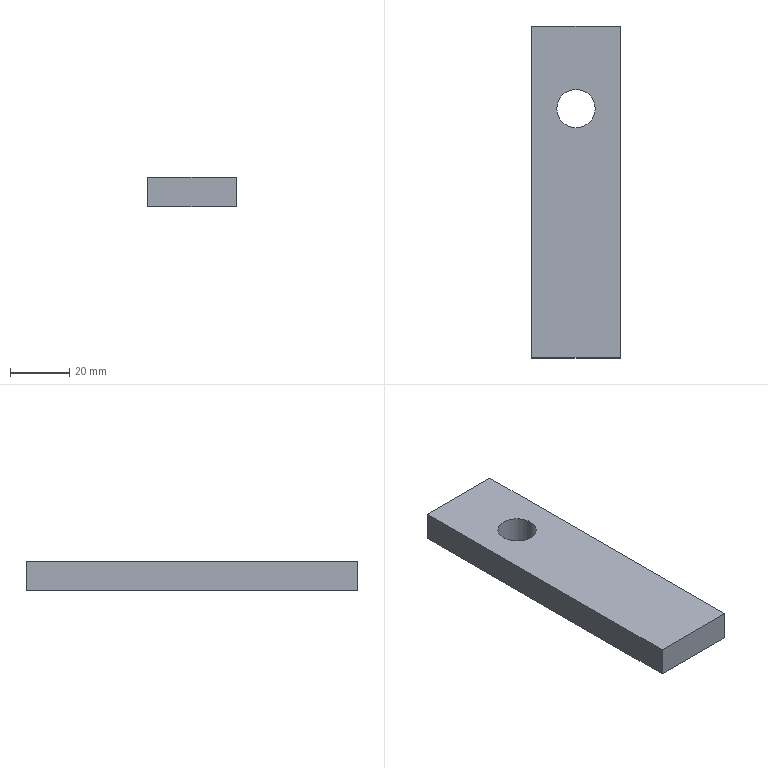Part | NX | features solid 2 | 1 solid | 7 faces | box 30 x 112.5 x 10 mm | volume 32423 mm3 | plane 6 | cylinder 1 | commonest cylinder face diameters 13 x1
STEP:
#1=CARTESIAN_POINT('',(-15.,825.,-115.));
#2=VERTEX_POINT('',#1);
#3=CARTESIAN_POINT('',(15.,825.,-115.));
#4=VERTEX_POINT('',#3);
#5=CARTESIAN_POINT('',(15.,825.,-115.));
#6=DIRECTION('',(-1.,0.,0.));
#7=VECTOR('',#6,1000.);
#8=LINE('',#5,#7);
#9=EDGE_CURVE('',#2,#4,#8,.F.);
#10=ORIENTED_EDGE('',*,*,#9,.F.);
#11=CARTESIAN_POINT('',(-15.,712.5,-115.));
#12=VERTEX_POINT('',#11);
#13=CARTESIAN_POINT('',(-15.,735.,-115.));
#14=DIRECTION('',(0.,1.,0.));
#15=VECTOR('',#14,1000.);
#16=LINE('',#13,#15);
#17=EDGE_CURVE('',#12,#2,#16,.T.);
#18=ORIENTED_EDGE('',*,*,#17,.F.);
#19=CARTESIAN_POINT('',(15.,712.5,-115.));
#20=VERTEX_POINT('',#19);
#21=CARTESIAN_POINT('',(15.,712.5,-115.));
#22=DIRECTION('',(-1.,0.,0.));
#23=VECTOR('',#22,1000.);
#24=LINE('',#21,#23);
#25=EDGE_CURVE('',#20,#12,#24,.T.);
#26=ORIENTED_EDGE('',*,*,#25,.F.);
#27=CARTESIAN_POINT('',(15.,895.,-115.));
#28=DIRECTION('',(0.,-1.,0.));
#29=VECTOR('',#28,1000.);
#30=LINE('',#27,#29);
#31=EDGE_CURVE('',#4,#20,#30,.T.);
#32=ORIENTED_EDGE('',*,*,#31,.F.);
#33=EDGE_LOOP('',(#10,#18,#26,#32));
#34=FACE_BOUND('',#33,.T.);
#35=CARTESIAN_POINT('',(-6.5,797.,-115.));
#36=VERTEX_POINT('',#35);
#37=CARTESIAN_POINT('',(0.,797.,-115.));
#38=DIRECTION('',(0.,0.,-1.));
#39=DIRECTION('',(-1.,0.,0.));
#40=AXIS2_PLACEMENT_3D('',#37,#38,#39);
#41=CIRCLE('',#40,6.5);
#42=EDGE_CURVE('',#36,#36,#41,.F.);
#43=ORIENTED_EDGE('',*,*,#42,.F.);
#44=EDGE_LOOP('',(#43));
#45=FACE_BOUND('',#44,.T.);
#46=CARTESIAN_POINT('',(15.,895.,-115.));
#47=DIRECTION('',(0.,0.,-1.));
#48=DIRECTION('',(-1.,0.,0.));
#49=AXIS2_PLACEMENT_3D('',#46,#47,#48);
#50=PLANE('',#49);
#51=ADVANCED_FACE('',(#34,#45),#50,.F.);
#52=CARTESIAN_POINT('',(-15.,825.,-125.));
#53=VERTEX_POINT('',#52);
#54=CARTESIAN_POINT('',(15.,825.,-125.));
#55=VERTEX_POINT('',#54);
#56=CARTESIAN_POINT('',(15.,825.,-125.));
#57=DIRECTION('',(-1.,0.,0.));
#58=VECTOR('',#57,1000.);
#59=LINE('',#56,#58);
#60=EDGE_CURVE('',#53,#55,#59,.F.);
#61=ORIENTED_EDGE('',*,*,#60,.T.);
#62=CARTESIAN_POINT('',(15.,712.5,-125.));
#63=VERTEX_POINT('',#62);
#64=CARTESIAN_POINT('',(15.,895.,-125.));
#65=DIRECTION('',(0.,-1.,0.));
#66=VECTOR('',#65,1000.);
#67=LINE('',#64,#66);
#68=EDGE_CURVE('',#55,#63,#67,.T.);
#69=ORIENTED_EDGE('',*,*,#68,.T.);
#70=CARTESIAN_POINT('',(-15.,712.5,-125.));
#71=VERTEX_POINT('',#70);
#72=CARTESIAN_POINT('',(15.,712.5,-125.));
#73=DIRECTION('',(-1.,0.,0.));
#74=VECTOR('',#73,1000.);
#75=LINE('',#72,#74);
#76=EDGE_CURVE('',#63,#71,#75,.T.);
#77=ORIENTED_EDGE('',*,*,#76,.T.);
#78=CARTESIAN_POINT('',(-15.,735.,-125.));
#79=DIRECTION('',(0.,1.,0.));
#80=VECTOR('',#79,1000.);
#81=LINE('',#78,#80);
#82=EDGE_CURVE('',#71,#53,#81,.T.);
#83=ORIENTED_EDGE('',*,*,#82,.T.);
#84=EDGE_LOOP('',(#61,#69,#77,#83));
#85=FACE_BOUND('',#84,.T.);
#86=CARTESIAN_POINT('',(-6.5,797.,-125.));
#87=VERTEX_POINT('',#86);
#88=CARTESIAN_POINT('',(0.,797.,-125.));
#89=DIRECTION('',(0.,0.,-1.));
#90=DIRECTION('',(-1.,0.,0.));
#91=AXIS2_PLACEMENT_3D('',#88,#89,#90);
#92=CIRCLE('',#91,6.5);
#93=EDGE_CURVE('',#87,#87,#92,.F.);
#94=ORIENTED_EDGE('',*,*,#93,.T.);
#95=EDGE_LOOP('',(#94));
#96=FACE_BOUND('',#95,.T.);
#97=CARTESIAN_POINT('',(15.,895.,-125.));
#98=DIRECTION('',(0.,0.,-1.));
#99=DIRECTION('',(-1.,0.,0.));
#100=AXIS2_PLACEMENT_3D('',#97,#98,#99);
#101=PLANE('',#100);
#102=ADVANCED_FACE('',(#85,#96),#101,.T.);
#103=ORIENTED_EDGE('',*,*,#60,.F.);
#104=CARTESIAN_POINT('',(-15.,825.,-115.));
#105=DIRECTION('',(0.,0.,1.));
#106=VECTOR('',#105,1000.);
#107=LINE('',#104,#106);
#108=EDGE_CURVE('',#2,#53,#107,.F.);
#109=ORIENTED_EDGE('',*,*,#108,.F.);
#110=ORIENTED_EDGE('',*,*,#9,.T.);
#111=CARTESIAN_POINT('',(15.,825.,-180.));
#112=DIRECTION('',(0.,0.,1.));
#113=VECTOR('',#112,1000.);
#114=LINE('',#111,#113);
#115=EDGE_CURVE('',#4,#55,#114,.F.);
#116=ORIENTED_EDGE('',*,*,#115,.T.);
#117=EDGE_LOOP('',(#103,#109,#110,#116));
#118=FACE_BOUND('',#117,.T.);
#119=CARTESIAN_POINT('',(-28.,825.,-180.));
#120=DIRECTION('',(0.,-1.,0.));
#121=DIRECTION('',(0.,0.,-1.));
#122=AXIS2_PLACEMENT_3D('',#119,#120,#121);
#123=PLANE('',#122);
#124=ADVANCED_FACE('',(#118),#123,.F.);
#125=ORIENTED_EDGE('',*,*,#68,.F.);
#126=ORIENTED_EDGE('',*,*,#115,.F.);
#127=ORIENTED_EDGE('',*,*,#31,.T.);
#128=CARTESIAN_POINT('',(15.,712.5,-115.));
#129=DIRECTION('',(0.,0.,-1.));
#130=VECTOR('',#129,1000.);
#131=LINE('',#128,#130);
#132=EDGE_CURVE('',#20,#63,#131,.T.);
#133=ORIENTED_EDGE('',*,*,#132,.T.);
#134=EDGE_LOOP('',(#125,#126,#127,#133));
#135=FACE_BOUND('',#134,.T.);
#136=CARTESIAN_POINT('',(15.,895.,-115.));
#137=DIRECTION('',(1.,0.,0.));
#138=DIRECTION('',(0.,0.,-1.));
#139=AXIS2_PLACEMENT_3D('',#136,#137,#138);
#140=PLANE('',#139);
#141=ADVANCED_FACE('',(#135),#140,.T.);
#142=ORIENTED_EDGE('',*,*,#76,.F.);
#143=ORIENTED_EDGE('',*,*,#132,.F.);
#144=ORIENTED_EDGE('',*,*,#25,.T.);
#145=CARTESIAN_POINT('',(-15.,712.5,-101.));
#146=DIRECTION('',(0.,0.,-1.));
#147=VECTOR('',#146,1000.);
#148=LINE('',#145,#147);
#149=EDGE_CURVE('',#12,#71,#148,.T.);
#150=ORIENTED_EDGE('',*,*,#149,.T.);
#151=EDGE_LOOP('',(#142,#143,#144,#150));
#152=FACE_BOUND('',#151,.T.);
#153=CARTESIAN_POINT('',(10.,712.5,-101.));
#154=DIRECTION('',(0.,-1.,0.));
#155=DIRECTION('',(0.,0.,-1.));
#156=AXIS2_PLACEMENT_3D('',#153,#154,#155);
#157=PLANE('',#156);
#158=ADVANCED_FACE('',(#152),#157,.T.);
#159=ORIENTED_EDGE('',*,*,#82,.F.);
#160=ORIENTED_EDGE('',*,*,#149,.F.);
#161=ORIENTED_EDGE('',*,*,#17,.T.);
#162=ORIENTED_EDGE('',*,*,#108,.T.);
#163=EDGE_LOOP('',(#159,#160,#161,#162));
#164=FACE_BOUND('',#163,.T.);
#165=CARTESIAN_POINT('',(-15.,735.,-115.));
#166=DIRECTION('',(-1.,0.,0.));
#167=DIRECTION('',(0.,0.,1.));
#168=AXIS2_PLACEMENT_3D('',#165,#166,#167);
#169=PLANE('',#168);
#170=ADVANCED_FACE('',(#164),#169,.T.);
#171=ORIENTED_EDGE('',*,*,#93,.F.);
#172=EDGE_LOOP('',(#171));
#173=FACE_BOUND('',#172,.T.);
#174=ORIENTED_EDGE('',*,*,#42,.T.);
#175=EDGE_LOOP('',(#174));
#176=FACE_BOUND('',#175,.T.);
#177=CARTESIAN_POINT('',(0.,797.,-1.));
#178=DIRECTION('',(0.,0.,-1.));
#179=DIRECTION('',(-1.,0.,0.));
#180=AXIS2_PLACEMENT_3D('',#177,#178,#179);
#181=CYLINDRICAL_SURFACE('',#180,6.5);
#182=ADVANCED_FACE('',(#173,#176),#181,.F.);
#183=CLOSED_SHELL('',(#51,#102,#124,#141,#158,#170,#182));
#184=MANIFOLD_SOLID_BREP('',#183);
#185=(LENGTH_UNIT()NAMED_UNIT(*)SI_UNIT(.MILLI.,.METRE.));
#186=UNCERTAINTY_MEASURE_WITH_UNIT(LENGTH_MEASURE(0.00001),#185,'','');
#187=(NAMED_UNIT(*)PLANE_ANGLE_UNIT()SI_UNIT($,.RADIAN.));
#188=(NAMED_UNIT(*)SI_UNIT($,.STERADIAN.)SOLID_ANGLE_UNIT());
#189=(GEOMETRIC_REPRESENTATION_CONTEXT(3)GLOBAL_UNCERTAINTY_ASSIGNED_CONTEXT((#186))GLOBAL_UNIT_ASSIGNED_CONTEXT((#185,#187,#188))REPRESENTATION_CONTEXT('',''));
#190=ADVANCED_BREP_SHAPE_REPRESENTATION('',(#184),#189);